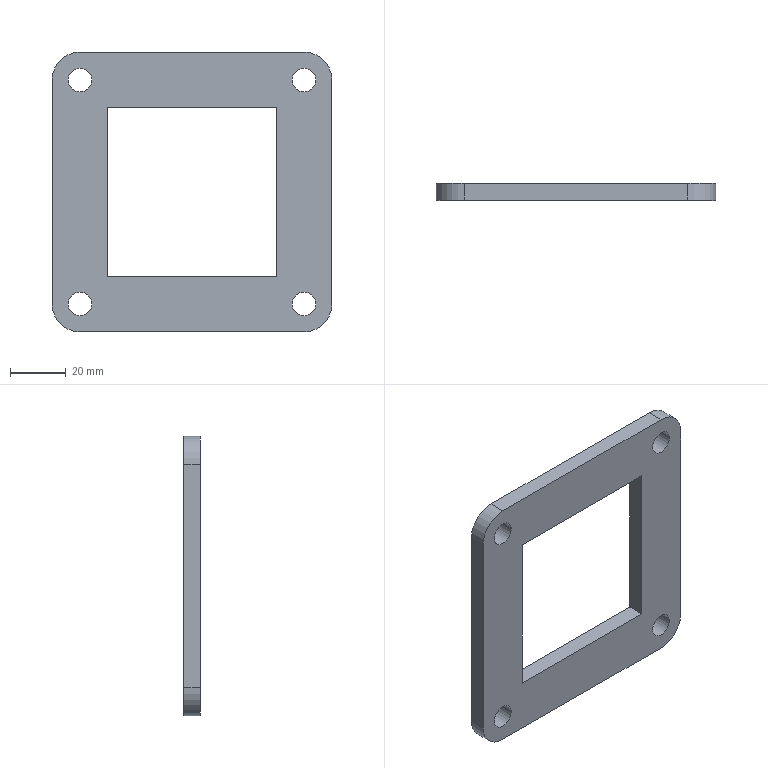Part | STEP file | JBJ-P-1013-02 | 1 solid | 18 faces | box 100 x 6 x 100 mm | volume 36162 mm3 | plane 10 | cylinder 8 | commonest cylinder face diameters 8.5 x4 20 x4
STEP:
#1=CARTESIAN_POINT('',(0.,0.,10.));
#2=VERTEX_POINT('',#1);
#3=CARTESIAN_POINT('',(0.,0.,90.));
#4=VERTEX_POINT('',#3);
#5=CARTESIAN_POINT('',(0.,0.,0.));
#6=DIRECTION('',(0.,0.,1.));
#7=VECTOR('',#6,1000.);
#8=LINE('',#5,#7);
#9=EDGE_CURVE('',#2,#4,#8,.T.);
#10=ORIENTED_EDGE('',*,*,#9,.T.);
#11=CARTESIAN_POINT('',(0.,6.,90.));
#12=VERTEX_POINT('',#11);
#13=CARTESIAN_POINT('',(0.,6.,90.));
#14=DIRECTION('',(0.,1.,0.));
#15=VECTOR('',#14,1000.);
#16=LINE('',#13,#15);
#17=EDGE_CURVE('',#4,#12,#16,.T.);
#18=ORIENTED_EDGE('',*,*,#17,.T.);
#19=CARTESIAN_POINT('',(0.,6.,10.));
#20=VERTEX_POINT('',#19);
#21=CARTESIAN_POINT('',(0.,6.,0.));
#22=DIRECTION('',(0.,0.,1.));
#23=VECTOR('',#22,1000.);
#24=LINE('',#21,#23);
#25=EDGE_CURVE('',#20,#12,#24,.T.);
#26=ORIENTED_EDGE('',*,*,#25,.F.);
#27=CARTESIAN_POINT('',(0.,6.,10.));
#28=DIRECTION('',(0.,-1.,0.));
#29=VECTOR('',#28,1000.);
#30=LINE('',#27,#29);
#31=EDGE_CURVE('',#20,#2,#30,.T.);
#32=ORIENTED_EDGE('',*,*,#31,.T.);
#33=EDGE_LOOP('',(#10,#18,#26,#32));
#34=FACE_OUTER_BOUND('',#33,.T.);
#35=CARTESIAN_POINT('',(0.,6.,0.));
#36=DIRECTION('',(1.,0.,0.));
#37=DIRECTION('',(0.,0.,-1.));
#38=AXIS2_PLACEMENT_3D('',#35,#36,#37);
#39=PLANE('',#38);
#40=ADVANCED_FACE('',(#34),#39,.F.);
#41=CARTESIAN_POINT('',(10.,0.,100.));
#42=VERTEX_POINT('',#41);
#43=CARTESIAN_POINT('',(90.,0.,100.));
#44=VERTEX_POINT('',#43);
#45=CARTESIAN_POINT('',(0.,0.,100.));
#46=DIRECTION('',(1.,0.,0.));
#47=VECTOR('',#46,1000.);
#48=LINE('',#45,#47);
#49=EDGE_CURVE('',#42,#44,#48,.T.);
#50=ORIENTED_EDGE('',*,*,#49,.T.);
#51=CARTESIAN_POINT('',(90.,6.,100.));
#52=VERTEX_POINT('',#51);
#53=CARTESIAN_POINT('',(90.,6.,100.));
#54=DIRECTION('',(0.,1.,0.));
#55=VECTOR('',#54,1000.);
#56=LINE('',#53,#55);
#57=EDGE_CURVE('',#44,#52,#56,.T.);
#58=ORIENTED_EDGE('',*,*,#57,.T.);
#59=CARTESIAN_POINT('',(10.,6.,100.));
#60=VERTEX_POINT('',#59);
#61=CARTESIAN_POINT('',(0.,6.,100.));
#62=DIRECTION('',(1.,0.,0.));
#63=VECTOR('',#62,1000.);
#64=LINE('',#61,#63);
#65=EDGE_CURVE('',#60,#52,#64,.T.);
#66=ORIENTED_EDGE('',*,*,#65,.F.);
#67=CARTESIAN_POINT('',(10.,6.,100.));
#68=DIRECTION('',(0.,-1.,0.));
#69=VECTOR('',#68,1000.);
#70=LINE('',#67,#69);
#71=EDGE_CURVE('',#60,#42,#70,.T.);
#72=ORIENTED_EDGE('',*,*,#71,.T.);
#73=EDGE_LOOP('',(#50,#58,#66,#72));
#74=FACE_OUTER_BOUND('',#73,.T.);
#75=CARTESIAN_POINT('',(0.,6.,100.));
#76=DIRECTION('',(0.,0.,-1.));
#77=DIRECTION('',(-1.,0.,0.));
#78=AXIS2_PLACEMENT_3D('',#75,#76,#77);
#79=PLANE('',#78);
#80=ADVANCED_FACE('',(#74),#79,.F.);
#81=CARTESIAN_POINT('',(100.,6.,90.));
#82=VERTEX_POINT('',#81);
#83=CARTESIAN_POINT('',(100.,6.,10.));
#84=VERTEX_POINT('',#83);
#85=CARTESIAN_POINT('',(100.,6.,0.));
#86=DIRECTION('',(0.,0.,-1.));
#87=VECTOR('',#86,1000.);
#88=LINE('',#85,#87);
#89=EDGE_CURVE('',#82,#84,#88,.T.);
#90=ORIENTED_EDGE('',*,*,#89,.F.);
#91=CARTESIAN_POINT('',(100.,0.,90.));
#92=VERTEX_POINT('',#91);
#93=CARTESIAN_POINT('',(100.,6.,90.));
#94=DIRECTION('',(0.,-1.,0.));
#95=VECTOR('',#94,1000.);
#96=LINE('',#93,#95);
#97=EDGE_CURVE('',#82,#92,#96,.T.);
#98=ORIENTED_EDGE('',*,*,#97,.T.);
#99=CARTESIAN_POINT('',(100.,0.,10.));
#100=VERTEX_POINT('',#99);
#101=CARTESIAN_POINT('',(100.,0.,0.));
#102=DIRECTION('',(0.,0.,-1.));
#103=VECTOR('',#102,1000.);
#104=LINE('',#101,#103);
#105=EDGE_CURVE('',#92,#100,#104,.T.);
#106=ORIENTED_EDGE('',*,*,#105,.T.);
#107=CARTESIAN_POINT('',(100.,6.,10.));
#108=DIRECTION('',(0.,1.,0.));
#109=VECTOR('',#108,1000.);
#110=LINE('',#107,#109);
#111=EDGE_CURVE('',#100,#84,#110,.T.);
#112=ORIENTED_EDGE('',*,*,#111,.T.);
#113=EDGE_LOOP('',(#90,#98,#106,#112));
#114=FACE_OUTER_BOUND('',#113,.T.);
#115=CARTESIAN_POINT('',(100.,6.,0.));
#116=DIRECTION('',(-1.,0.,0.));
#117=DIRECTION('',(0.,0.,1.));
#118=AXIS2_PLACEMENT_3D('',#115,#116,#117);
#119=PLANE('',#118);
#120=ADVANCED_FACE('',(#114),#119,.F.);
#121=CARTESIAN_POINT('',(90.,6.,0.));
#122=VERTEX_POINT('',#121);
#123=CARTESIAN_POINT('',(10.,6.,0.));
#124=VERTEX_POINT('',#123);
#125=CARTESIAN_POINT('',(0.,6.,0.));
#126=DIRECTION('',(-1.,0.,0.));
#127=VECTOR('',#126,1000.);
#128=LINE('',#125,#127);
#129=EDGE_CURVE('',#122,#124,#128,.T.);
#130=ORIENTED_EDGE('',*,*,#129,.F.);
#131=CARTESIAN_POINT('',(90.,0.,0.));
#132=VERTEX_POINT('',#131);
#133=CARTESIAN_POINT('',(90.,6.,0.));
#134=DIRECTION('',(0.,-1.,0.));
#135=VECTOR('',#134,1000.);
#136=LINE('',#133,#135);
#137=EDGE_CURVE('',#122,#132,#136,.T.);
#138=ORIENTED_EDGE('',*,*,#137,.T.);
#139=CARTESIAN_POINT('',(10.,0.,0.));
#140=VERTEX_POINT('',#139);
#141=CARTESIAN_POINT('',(0.,0.,0.));
#142=DIRECTION('',(-1.,0.,0.));
#143=VECTOR('',#142,1000.);
#144=LINE('',#141,#143);
#145=EDGE_CURVE('',#132,#140,#144,.T.);
#146=ORIENTED_EDGE('',*,*,#145,.T.);
#147=CARTESIAN_POINT('',(10.,6.,0.));
#148=DIRECTION('',(0.,1.,0.));
#149=VECTOR('',#148,1000.);
#150=LINE('',#147,#149);
#151=EDGE_CURVE('',#140,#124,#150,.T.);
#152=ORIENTED_EDGE('',*,*,#151,.T.);
#153=EDGE_LOOP('',(#130,#138,#146,#152));
#154=FACE_OUTER_BOUND('',#153,.T.);
#155=CARTESIAN_POINT('',(0.,6.,0.));
#156=DIRECTION('',(0.,0.,1.));
#157=DIRECTION('',(1.,0.,0.));
#158=AXIS2_PLACEMENT_3D('',#155,#156,#157);
#159=PLANE('',#158);
#160=ADVANCED_FACE('',(#154),#159,.F.);
#161=CARTESIAN_POINT('',(80.25,6.,80.25));
#162=VERTEX_POINT('',#161);
#163=CARTESIAN_POINT('',(80.25,6.,19.75));
#164=VERTEX_POINT('',#163);
#165=CARTESIAN_POINT('',(80.25,6.,19.75));
#166=DIRECTION('',(0.,0.,-1.));
#167=VECTOR('',#166,1000.);
#168=LINE('',#165,#167);
#169=EDGE_CURVE('',#162,#164,#168,.T.);
#170=ORIENTED_EDGE('',*,*,#169,.F.);
#171=CARTESIAN_POINT('',(19.75,6.,80.25));
#172=VERTEX_POINT('',#171);
#173=CARTESIAN_POINT('',(19.75,6.,80.25));
#174=DIRECTION('',(1.,0.,0.));
#175=VECTOR('',#174,1000.);
#176=LINE('',#173,#175);
#177=EDGE_CURVE('',#172,#162,#176,.T.);
#178=ORIENTED_EDGE('',*,*,#177,.F.);
#179=CARTESIAN_POINT('',(19.75,6.,19.75));
#180=VERTEX_POINT('',#179);
#181=CARTESIAN_POINT('',(19.75,6.,19.75));
#182=DIRECTION('',(0.,0.,1.));
#183=VECTOR('',#182,1000.);
#184=LINE('',#181,#183);
#185=EDGE_CURVE('',#180,#172,#184,.T.);
#186=ORIENTED_EDGE('',*,*,#185,.F.);
#187=CARTESIAN_POINT('',(19.75,6.,19.75));
#188=DIRECTION('',(-1.,0.,0.));
#189=VECTOR('',#188,1000.);
#190=LINE('',#187,#189);
#191=EDGE_CURVE('',#164,#180,#190,.T.);
#192=ORIENTED_EDGE('',*,*,#191,.F.);
#193=EDGE_LOOP('',(#170,#178,#186,#192));
#194=FACE_BOUND('',#193,.T.);
#195=CARTESIAN_POINT('',(10.,6.,14.25));
#196=VERTEX_POINT('',#195);
#197=CARTESIAN_POINT('',(10.,6.,10.));
#198=DIRECTION('',(0.,1.,0.));
#199=DIRECTION('',(0.,0.,1.));
#200=AXIS2_PLACEMENT_3D('',#197,#198,#199);
#201=CIRCLE('',#200,4.25);
#202=EDGE_CURVE('',#196,#196,#201,.T.);
#203=ORIENTED_EDGE('',*,*,#202,.F.);
#204=EDGE_LOOP('',(#203));
#205=FACE_BOUND('',#204,.T.);
#206=CARTESIAN_POINT('',(90.,6.,14.25));
#207=VERTEX_POINT('',#206);
#208=CARTESIAN_POINT('',(90.,6.,10.));
#209=DIRECTION('',(0.,1.,0.));
#210=DIRECTION('',(0.,0.,1.));
#211=AXIS2_PLACEMENT_3D('',#208,#209,#210);
#212=CIRCLE('',#211,4.25);
#213=EDGE_CURVE('',#207,#207,#212,.T.);
#214=ORIENTED_EDGE('',*,*,#213,.F.);
#215=EDGE_LOOP('',(#214));
#216=FACE_BOUND('',#215,.T.);
#217=CARTESIAN_POINT('',(90.,6.,94.25));
#218=VERTEX_POINT('',#217);
#219=CARTESIAN_POINT('',(90.,6.,90.));
#220=DIRECTION('',(0.,1.,0.));
#221=DIRECTION('',(0.,0.,1.));
#222=AXIS2_PLACEMENT_3D('',#219,#220,#221);
#223=CIRCLE('',#222,4.25);
#224=EDGE_CURVE('',#218,#218,#223,.T.);
#225=ORIENTED_EDGE('',*,*,#224,.F.);
#226=EDGE_LOOP('',(#225));
#227=FACE_BOUND('',#226,.T.);
#228=CARTESIAN_POINT('',(10.,6.,94.25));
#229=VERTEX_POINT('',#228);
#230=CARTESIAN_POINT('',(10.,6.,90.));
#231=DIRECTION('',(0.,1.,0.));
#232=DIRECTION('',(0.,0.,1.));
#233=AXIS2_PLACEMENT_3D('',#230,#231,#232);
#234=CIRCLE('',#233,4.25);
#235=EDGE_CURVE('',#229,#229,#234,.T.);
#236=ORIENTED_EDGE('',*,*,#235,.F.);
#237=EDGE_LOOP('',(#236));
#238=FACE_BOUND('',#237,.T.);
#239=ORIENTED_EDGE('',*,*,#65,.T.);
#240=CARTESIAN_POINT('',(90.,6.,90.));
#241=DIRECTION('',(0.,1.,0.));
#242=DIRECTION('',(0.,0.,1.));
#243=AXIS2_PLACEMENT_3D('',#240,#241,#242);
#244=CIRCLE('',#243,10.);
#245=EDGE_CURVE('',#52,#82,#244,.T.);
#246=ORIENTED_EDGE('',*,*,#245,.T.);
#247=ORIENTED_EDGE('',*,*,#89,.T.);
#248=CARTESIAN_POINT('',(90.,6.,10.));
#249=DIRECTION('',(0.,1.,0.));
#250=DIRECTION('',(0.,0.,1.));
#251=AXIS2_PLACEMENT_3D('',#248,#249,#250);
#252=CIRCLE('',#251,10.);
#253=EDGE_CURVE('',#84,#122,#252,.T.);
#254=ORIENTED_EDGE('',*,*,#253,.T.);
#255=ORIENTED_EDGE('',*,*,#129,.T.);
#256=CARTESIAN_POINT('',(10.,6.,10.));
#257=DIRECTION('',(0.,1.,0.));
#258=DIRECTION('',(0.,0.,1.));
#259=AXIS2_PLACEMENT_3D('',#256,#257,#258);
#260=CIRCLE('',#259,10.);
#261=EDGE_CURVE('',#124,#20,#260,.T.);
#262=ORIENTED_EDGE('',*,*,#261,.T.);
#263=ORIENTED_EDGE('',*,*,#25,.T.);
#264=CARTESIAN_POINT('',(10.,6.,90.));
#265=DIRECTION('',(0.,1.,0.));
#266=DIRECTION('',(0.,0.,1.));
#267=AXIS2_PLACEMENT_3D('',#264,#265,#266);
#268=CIRCLE('',#267,10.);
#269=EDGE_CURVE('',#12,#60,#268,.T.);
#270=ORIENTED_EDGE('',*,*,#269,.T.);
#271=EDGE_LOOP('',(#239,#246,#247,#254,#255,#262,#263,#270));
#272=FACE_OUTER_BOUND('',#271,.T.);
#273=CARTESIAN_POINT('',(0.,6.,0.));
#274=DIRECTION('',(0.,1.,0.));
#275=DIRECTION('',(0.,0.,1.));
#276=AXIS2_PLACEMENT_3D('',#273,#274,#275);
#277=PLANE('',#276);
#278=ADVANCED_FACE('',(#194,#205,#216,#227,#238,#272),#277,.T.);
#279=CARTESIAN_POINT('',(19.75,0.,80.25));
#280=VERTEX_POINT('',#279);
#281=CARTESIAN_POINT('',(80.25,0.,80.25));
#282=VERTEX_POINT('',#281);
#283=CARTESIAN_POINT('',(19.75,0.,80.25));
#284=DIRECTION('',(1.,0.,0.));
#285=VECTOR('',#284,1000.);
#286=LINE('',#283,#285);
#287=EDGE_CURVE('',#280,#282,#286,.T.);
#288=ORIENTED_EDGE('',*,*,#287,.T.);
#289=CARTESIAN_POINT('',(80.25,0.,19.75));
#290=VERTEX_POINT('',#289);
#291=CARTESIAN_POINT('',(80.25,0.,19.75));
#292=DIRECTION('',(0.,0.,-1.));
#293=VECTOR('',#292,1000.);
#294=LINE('',#291,#293);
#295=EDGE_CURVE('',#282,#290,#294,.T.);
#296=ORIENTED_EDGE('',*,*,#295,.T.);
#297=CARTESIAN_POINT('',(19.75,0.,19.75));
#298=VERTEX_POINT('',#297);
#299=CARTESIAN_POINT('',(19.75,0.,19.75));
#300=DIRECTION('',(-1.,0.,0.));
#301=VECTOR('',#300,1000.);
#302=LINE('',#299,#301);
#303=EDGE_CURVE('',#290,#298,#302,.T.);
#304=ORIENTED_EDGE('',*,*,#303,.T.);
#305=CARTESIAN_POINT('',(19.75,0.,19.75));
#306=DIRECTION('',(0.,0.,1.));
#307=VECTOR('',#306,1000.);
#308=LINE('',#305,#307);
#309=EDGE_CURVE('',#298,#280,#308,.T.);
#310=ORIENTED_EDGE('',*,*,#309,.T.);
#311=EDGE_LOOP('',(#288,#296,#304,#310));
#312=FACE_BOUND('',#311,.T.);
#313=CARTESIAN_POINT('',(10.,0.,14.25));
#314=VERTEX_POINT('',#313);
#315=CARTESIAN_POINT('',(10.,0.,10.));
#316=DIRECTION('',(0.,1.,0.));
#317=DIRECTION('',(0.,0.,1.));
#318=AXIS2_PLACEMENT_3D('',#315,#316,#317);
#319=CIRCLE('',#318,4.25);
#320=EDGE_CURVE('',#314,#314,#319,.T.);
#321=ORIENTED_EDGE('',*,*,#320,.T.);
#322=EDGE_LOOP('',(#321));
#323=FACE_BOUND('',#322,.T.);
#324=CARTESIAN_POINT('',(90.,0.,14.25));
#325=VERTEX_POINT('',#324);
#326=CARTESIAN_POINT('',(90.,0.,10.));
#327=DIRECTION('',(0.,1.,0.));
#328=DIRECTION('',(0.,0.,1.));
#329=AXIS2_PLACEMENT_3D('',#326,#327,#328);
#330=CIRCLE('',#329,4.25);
#331=EDGE_CURVE('',#325,#325,#330,.T.);
#332=ORIENTED_EDGE('',*,*,#331,.T.);
#333=EDGE_LOOP('',(#332));
#334=FACE_BOUND('',#333,.T.);
#335=CARTESIAN_POINT('',(90.,0.,94.25));
#336=VERTEX_POINT('',#335);
#337=CARTESIAN_POINT('',(90.,0.,90.));
#338=DIRECTION('',(0.,1.,0.));
#339=DIRECTION('',(0.,0.,1.));
#340=AXIS2_PLACEMENT_3D('',#337,#338,#339);
#341=CIRCLE('',#340,4.25);
#342=EDGE_CURVE('',#336,#336,#341,.T.);
#343=ORIENTED_EDGE('',*,*,#342,.T.);
#344=EDGE_LOOP('',(#343));
#345=FACE_BOUND('',#344,.T.);
#346=CARTESIAN_POINT('',(10.,0.,94.25));
#347=VERTEX_POINT('',#346);
#348=CARTESIAN_POINT('',(10.,0.,90.));
#349=DIRECTION('',(0.,1.,0.));
#350=DIRECTION('',(0.,0.,1.));
#351=AXIS2_PLACEMENT_3D('',#348,#349,#350);
#352=CIRCLE('',#351,4.25);
#353=EDGE_CURVE('',#347,#347,#352,.T.);
#354=ORIENTED_EDGE('',*,*,#353,.T.);
#355=EDGE_LOOP('',(#354));
#356=FACE_BOUND('',#355,.T.);
#357=ORIENTED_EDGE('',*,*,#105,.F.);
#358=CARTESIAN_POINT('',(90.,0.,90.));
#359=DIRECTION('',(0.,-1.,0.));
#360=DIRECTION('',(0.,0.,1.));
#361=AXIS2_PLACEMENT_3D('',#358,#359,#360);
#362=CIRCLE('',#361,10.);
#363=EDGE_CURVE('',#92,#44,#362,.T.);
#364=ORIENTED_EDGE('',*,*,#363,.T.);
#365=ORIENTED_EDGE('',*,*,#49,.F.);
#366=CARTESIAN_POINT('',(10.,0.,90.));
#367=DIRECTION('',(0.,-1.,0.));
#368=DIRECTION('',(0.,0.,1.));
#369=AXIS2_PLACEMENT_3D('',#366,#367,#368);
#370=CIRCLE('',#369,10.);
#371=EDGE_CURVE('',#42,#4,#370,.T.);
#372=ORIENTED_EDGE('',*,*,#371,.T.);
#373=ORIENTED_EDGE('',*,*,#9,.F.);
#374=CARTESIAN_POINT('',(10.,0.,10.));
#375=DIRECTION('',(0.,-1.,0.));
#376=DIRECTION('',(0.,0.,1.));
#377=AXIS2_PLACEMENT_3D('',#374,#375,#376);
#378=CIRCLE('',#377,10.);
#379=EDGE_CURVE('',#2,#140,#378,.T.);
#380=ORIENTED_EDGE('',*,*,#379,.T.);
#381=ORIENTED_EDGE('',*,*,#145,.F.);
#382=CARTESIAN_POINT('',(90.,0.,10.));
#383=DIRECTION('',(0.,-1.,0.));
#384=DIRECTION('',(0.,0.,1.));
#385=AXIS2_PLACEMENT_3D('',#382,#383,#384);
#386=CIRCLE('',#385,10.);
#387=EDGE_CURVE('',#132,#100,#386,.T.);
#388=ORIENTED_EDGE('',*,*,#387,.T.);
#389=EDGE_LOOP('',(#357,#364,#365,#372,#373,#380,#381,#388));
#390=FACE_OUTER_BOUND('',#389,.T.);
#391=CARTESIAN_POINT('',(0.,0.,0.));
#392=DIRECTION('',(0.,1.,0.));
#393=DIRECTION('',(0.,0.,1.));
#394=AXIS2_PLACEMENT_3D('',#391,#392,#393);
#395=PLANE('',#394);
#396=ADVANCED_FACE('',(#312,#323,#334,#345,#356,#390),#395,.F.);
#397=ORIENTED_EDGE('',*,*,#353,.F.);
#398=EDGE_LOOP('',(#397));
#399=FACE_OUTER_BOUND('',#398,.T.);
#400=ORIENTED_EDGE('',*,*,#235,.T.);
#401=EDGE_LOOP('',(#400));
#402=FACE_OUTER_BOUND('',#401,.T.);
#403=CARTESIAN_POINT('',(10.,6.,90.));
#404=DIRECTION('',(0.,1.,0.));
#405=DIRECTION('',(0.,0.,1.));
#406=AXIS2_PLACEMENT_3D('',#403,#404,#405);
#407=CYLINDRICAL_SURFACE('',#406,4.25);
#408=ADVANCED_FACE('',(#399,#402),#407,.F.);
#409=ORIENTED_EDGE('',*,*,#342,.F.);
#410=EDGE_LOOP('',(#409));
#411=FACE_OUTER_BOUND('',#410,.T.);
#412=ORIENTED_EDGE('',*,*,#224,.T.);
#413=EDGE_LOOP('',(#412));
#414=FACE_OUTER_BOUND('',#413,.T.);
#415=CARTESIAN_POINT('',(90.,6.,90.));
#416=DIRECTION('',(0.,1.,0.));
#417=DIRECTION('',(0.,0.,1.));
#418=AXIS2_PLACEMENT_3D('',#415,#416,#417);
#419=CYLINDRICAL_SURFACE('',#418,4.25);
#420=ADVANCED_FACE('',(#411,#414),#419,.F.);
#421=ORIENTED_EDGE('',*,*,#331,.F.);
#422=EDGE_LOOP('',(#421));
#423=FACE_OUTER_BOUND('',#422,.T.);
#424=ORIENTED_EDGE('',*,*,#213,.T.);
#425=EDGE_LOOP('',(#424));
#426=FACE_OUTER_BOUND('',#425,.T.);
#427=CARTESIAN_POINT('',(90.,6.,10.));
#428=DIRECTION('',(0.,1.,0.));
#429=DIRECTION('',(0.,0.,1.));
#430=AXIS2_PLACEMENT_3D('',#427,#428,#429);
#431=CYLINDRICAL_SURFACE('',#430,4.25);
#432=ADVANCED_FACE('',(#423,#426),#431,.F.);
#433=ORIENTED_EDGE('',*,*,#320,.F.);
#434=EDGE_LOOP('',(#433));
#435=FACE_OUTER_BOUND('',#434,.T.);
#436=ORIENTED_EDGE('',*,*,#202,.T.);
#437=EDGE_LOOP('',(#436));
#438=FACE_OUTER_BOUND('',#437,.T.);
#439=CARTESIAN_POINT('',(10.,6.,10.));
#440=DIRECTION('',(0.,1.,0.));
#441=DIRECTION('',(0.,0.,1.));
#442=AXIS2_PLACEMENT_3D('',#439,#440,#441);
#443=CYLINDRICAL_SURFACE('',#442,4.25);
#444=ADVANCED_FACE('',(#435,#438),#443,.F.);
#445=ORIENTED_EDGE('',*,*,#245,.F.);
#446=ORIENTED_EDGE('',*,*,#57,.F.);
#447=ORIENTED_EDGE('',*,*,#363,.F.);
#448=ORIENTED_EDGE('',*,*,#97,.F.);
#449=EDGE_LOOP('',(#445,#446,#447,#448));
#450=FACE_OUTER_BOUND('',#449,.T.);
#451=CARTESIAN_POINT('',(90.,6.,90.));
#452=DIRECTION('',(0.,-1.,0.));
#453=DIRECTION('',(0.,0.,-1.));
#454=AXIS2_PLACEMENT_3D('',#451,#452,#453);
#455=CYLINDRICAL_SURFACE('',#454,10.);
#456=ADVANCED_FACE('',(#450),#455,.T.);
#457=ORIENTED_EDGE('',*,*,#269,.F.);
#458=ORIENTED_EDGE('',*,*,#17,.F.);
#459=ORIENTED_EDGE('',*,*,#371,.F.);
#460=ORIENTED_EDGE('',*,*,#71,.F.);
#461=EDGE_LOOP('',(#457,#458,#459,#460));
#462=FACE_OUTER_BOUND('',#461,.T.);
#463=CARTESIAN_POINT('',(10.,6.,90.));
#464=DIRECTION('',(0.,-1.,0.));
#465=DIRECTION('',(0.,0.,-1.));
#466=AXIS2_PLACEMENT_3D('',#463,#464,#465);
#467=CYLINDRICAL_SURFACE('',#466,10.);
#468=ADVANCED_FACE('',(#462),#467,.T.);
#469=ORIENTED_EDGE('',*,*,#253,.F.);
#470=ORIENTED_EDGE('',*,*,#111,.F.);
#471=ORIENTED_EDGE('',*,*,#387,.F.);
#472=ORIENTED_EDGE('',*,*,#137,.F.);
#473=EDGE_LOOP('',(#469,#470,#471,#472));
#474=FACE_OUTER_BOUND('',#473,.T.);
#475=CARTESIAN_POINT('',(90.,6.,10.));
#476=DIRECTION('',(0.,-1.,0.));
#477=DIRECTION('',(0.,0.,-1.));
#478=AXIS2_PLACEMENT_3D('',#475,#476,#477);
#479=CYLINDRICAL_SURFACE('',#478,10.);
#480=ADVANCED_FACE('',(#474),#479,.T.);
#481=ORIENTED_EDGE('',*,*,#261,.F.);
#482=ORIENTED_EDGE('',*,*,#151,.F.);
#483=ORIENTED_EDGE('',*,*,#379,.F.);
#484=ORIENTED_EDGE('',*,*,#31,.F.);
#485=EDGE_LOOP('',(#481,#482,#483,#484));
#486=FACE_OUTER_BOUND('',#485,.T.);
#487=CARTESIAN_POINT('',(10.,6.,10.));
#488=DIRECTION('',(0.,-1.,0.));
#489=DIRECTION('',(0.,0.,-1.));
#490=AXIS2_PLACEMENT_3D('',#487,#488,#489);
#491=CYLINDRICAL_SURFACE('',#490,10.);
#492=ADVANCED_FACE('',(#486),#491,.T.);
#493=ORIENTED_EDGE('',*,*,#169,.T.);
#494=CARTESIAN_POINT('',(80.25,0.,19.75));
#495=DIRECTION('',(0.,1.,0.));
#496=VECTOR('',#495,1000.);
#497=LINE('',#494,#496);
#498=EDGE_CURVE('',#290,#164,#497,.T.);
#499=ORIENTED_EDGE('',*,*,#498,.F.);
#500=ORIENTED_EDGE('',*,*,#295,.F.);
#501=CARTESIAN_POINT('',(80.25,0.,80.25));
#502=DIRECTION('',(0.,1.,0.));
#503=VECTOR('',#502,1000.);
#504=LINE('',#501,#503);
#505=EDGE_CURVE('',#282,#162,#504,.T.);
#506=ORIENTED_EDGE('',*,*,#505,.T.);
#507=EDGE_LOOP('',(#493,#499,#500,#506));
#508=FACE_OUTER_BOUND('',#507,.T.);
#509=CARTESIAN_POINT('',(80.25,0.,19.75));
#510=DIRECTION('',(1.,0.,0.));
#511=DIRECTION('',(0.,0.,-1.));
#512=AXIS2_PLACEMENT_3D('',#509,#510,#511);
#513=PLANE('',#512);
#514=ADVANCED_FACE('',(#508),#513,.F.);
#515=ORIENTED_EDGE('',*,*,#177,.T.);
#516=ORIENTED_EDGE('',*,*,#505,.F.);
#517=ORIENTED_EDGE('',*,*,#287,.F.);
#518=CARTESIAN_POINT('',(19.75,0.,80.25));
#519=DIRECTION('',(0.,1.,0.));
#520=VECTOR('',#519,1000.);
#521=LINE('',#518,#520);
#522=EDGE_CURVE('',#280,#172,#521,.T.);
#523=ORIENTED_EDGE('',*,*,#522,.T.);
#524=EDGE_LOOP('',(#515,#516,#517,#523));
#525=FACE_OUTER_BOUND('',#524,.T.);
#526=CARTESIAN_POINT('',(19.75,0.,80.25));
#527=DIRECTION('',(0.,0.,1.));
#528=DIRECTION('',(1.,0.,0.));
#529=AXIS2_PLACEMENT_3D('',#526,#527,#528);
#530=PLANE('',#529);
#531=ADVANCED_FACE('',(#525),#530,.F.);
#532=ORIENTED_EDGE('',*,*,#185,.T.);
#533=ORIENTED_EDGE('',*,*,#522,.F.);
#534=ORIENTED_EDGE('',*,*,#309,.F.);
#535=CARTESIAN_POINT('',(19.75,0.,19.75));
#536=DIRECTION('',(0.,1.,0.));
#537=VECTOR('',#536,1000.);
#538=LINE('',#535,#537);
#539=EDGE_CURVE('',#298,#180,#538,.T.);
#540=ORIENTED_EDGE('',*,*,#539,.T.);
#541=EDGE_LOOP('',(#532,#533,#534,#540));
#542=FACE_OUTER_BOUND('',#541,.T.);
#543=CARTESIAN_POINT('',(19.75,0.,19.75));
#544=DIRECTION('',(-1.,0.,0.));
#545=DIRECTION('',(0.,0.,1.));
#546=AXIS2_PLACEMENT_3D('',#543,#544,#545);
#547=PLANE('',#546);
#548=ADVANCED_FACE('',(#542),#547,.F.);
#549=ORIENTED_EDGE('',*,*,#191,.T.);
#550=ORIENTED_EDGE('',*,*,#539,.F.);
#551=ORIENTED_EDGE('',*,*,#303,.F.);
#552=ORIENTED_EDGE('',*,*,#498,.T.);
#553=EDGE_LOOP('',(#549,#550,#551,#552));
#554=FACE_OUTER_BOUND('',#553,.T.);
#555=CARTESIAN_POINT('',(19.75,0.,19.75));
#556=DIRECTION('',(0.,0.,-1.));
#557=DIRECTION('',(-1.,0.,0.));
#558=AXIS2_PLACEMENT_3D('',#555,#556,#557);
#559=PLANE('',#558);
#560=ADVANCED_FACE('',(#554),#559,.F.);
#561=CLOSED_SHELL('',(#40,#80,#120,#160,#278,#396,#408,#420,#432,#444,#456,#468,#480,#492,#514,#531,#548,#560));
#562=MANIFOLD_SOLID_BREP('',#561);
#563=CARTESIAN_POINT('',(0.,0.,0.));
#564=DIRECTION('',(0.,0.,1.));
#565=DIRECTION('',(1.,0.,0.));
#566=AXIS2_PLACEMENT_3D('',#563,#564,#565);
#567=(LENGTH_UNIT()NAMED_UNIT(*)SI_UNIT(.MILLI.,.METRE.));
#568=UNCERTAINTY_MEASURE_WITH_UNIT(LENGTH_MEASURE(0.00001),#567,'','');
#569=(NAMED_UNIT(*)PLANE_ANGLE_UNIT()SI_UNIT($,.RADIAN.));
#570=(NAMED_UNIT(*)SI_UNIT($,.STERADIAN.)SOLID_ANGLE_UNIT());
#571=(GEOMETRIC_REPRESENTATION_CONTEXT(3)GLOBAL_UNCERTAINTY_ASSIGNED_CONTEXT((#568))GLOBAL_UNIT_ASSIGNED_CONTEXT((#567,#569,#570))REPRESENTATION_CONTEXT('',''));
#572=ADVANCED_BREP_SHAPE_REPRESENTATION('',(#562,#566),#571);